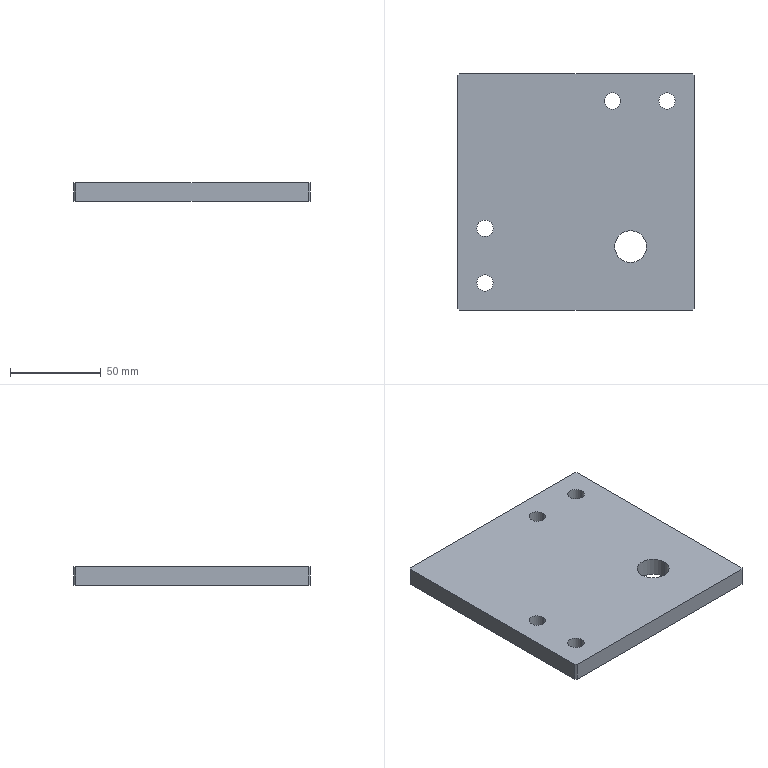Part | STEP file | Foot plate | 1 solid | 20 faces | box 130 x 130 x 10 mm | volume 164030 mm3 | cylinder 10 | plane 10 | commonest cylinder face diameters 9 x8 17.5 x2